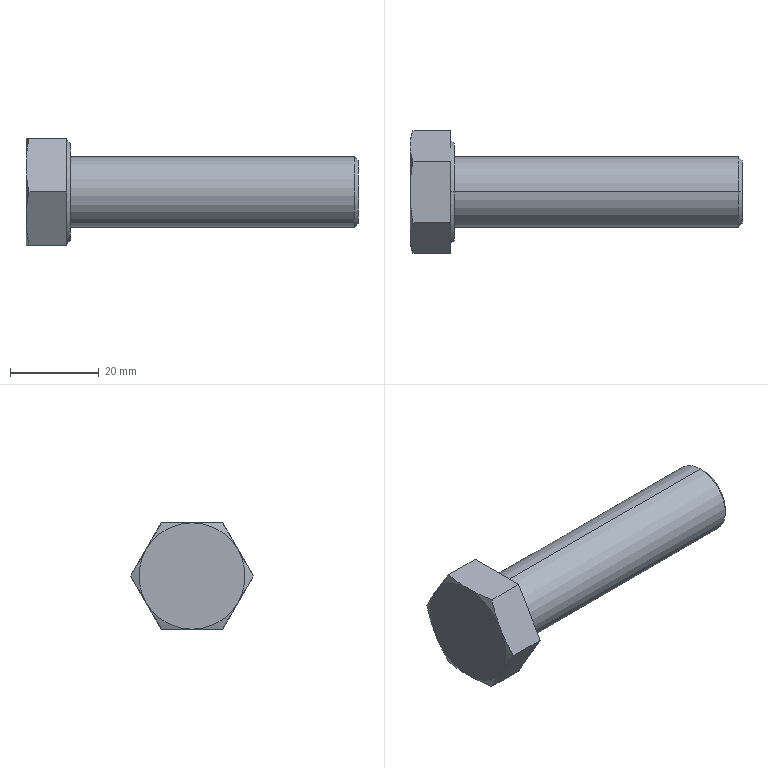Part | SolidWorks | features RevCut 3, Boss 1, Chamfer 1, Extrusion 1, Fillet 1, LPattern 1 | 1 solid | 22 faces | box 75 x 27.713 x 24 mm | volume 17960 mm3 | cone 10 | plane 10 | cylinder 2 | commonest cylinder face diameters 16 x2
STEP:
#1=CARTESIAN_POINT('',(75.,0.,-7.2));
#2=VERTEX_POINT('',#1);
#3=CARTESIAN_POINT('',(75.,0.,7.2));
#4=VERTEX_POINT('',#3);
#5=CARTESIAN_POINT('',(75.,0.,0.));
#6=DIRECTION('',(1.,0.,0.));
#7=DIRECTION('',(0.,0.,-1.));
#8=AXIS2_PLACEMENT_3D('',#5,#6,#7);
#9=CIRCLE('',#8,7.2);
#10=EDGE_CURVE('',#2,#4,#9,.T.);
#11=ORIENTED_EDGE('',*,*,#10,.F.);
#12=CARTESIAN_POINT('',(74.2,0.,-8.));
#13=VERTEX_POINT('',#12);
#14=CARTESIAN_POINT('',(75.,0.,-7.2));
#15=DIRECTION('',(-0.7071,0.,-0.7071));
#16=VECTOR('',#15,1000.);
#17=LINE('',#14,#16);
#18=EDGE_CURVE('',#2,#13,#17,.T.);
#19=ORIENTED_EDGE('',*,*,#18,.T.);
#20=CARTESIAN_POINT('',(74.2,0.,8.));
#21=VERTEX_POINT('',#20);
#22=CARTESIAN_POINT('',(74.2,0.,0.));
#23=DIRECTION('',(-1.,0.,0.));
#24=DIRECTION('',(0.,0.,-1.));
#25=AXIS2_PLACEMENT_3D('',#22,#23,#24);
#26=CIRCLE('',#25,8.);
#27=EDGE_CURVE('',#21,#13,#26,.T.);
#28=ORIENTED_EDGE('',*,*,#27,.F.);
#29=CARTESIAN_POINT('',(75.,0.,7.2));
#30=DIRECTION('',(-0.7071,0.,0.7071));
#31=VECTOR('',#30,1000.);
#32=LINE('',#29,#31);
#33=EDGE_CURVE('',#4,#21,#32,.T.);
#34=ORIENTED_EDGE('',*,*,#33,.F.);
#35=EDGE_LOOP('',(#11,#19,#28,#34));
#36=FACE_OUTER_BOUND('',#35,.T.);
#37=CARTESIAN_POINT('',(75.,0.,0.));
#38=DIRECTION('',(-1.,0.,0.));
#39=DIRECTION('',(0.,0.,1.));
#40=AXIS2_PLACEMENT_3D('',#37,#38,#39);
#41=CONICAL_SURFACE('',#40,7.2,0.7854);
#42=ADVANCED_FACE('',(#36),#41,.T.);
#43=ORIENTED_EDGE('',*,*,#27,.T.);
#44=CARTESIAN_POINT('',(10.,0.,-8.));
#45=VERTEX_POINT('',#44);
#46=CARTESIAN_POINT('',(75.,0.,-8.));
#47=DIRECTION('',(-1.,0.,0.));
#48=VECTOR('',#47,1000.);
#49=LINE('',#46,#48);
#50=EDGE_CURVE('',#13,#45,#49,.T.);
#51=ORIENTED_EDGE('',*,*,#50,.T.);
#52=CARTESIAN_POINT('',(10.,0.,8.));
#53=VERTEX_POINT('',#52);
#54=CARTESIAN_POINT('',(10.,0.,0.));
#55=DIRECTION('',(1.,0.,0.));
#56=DIRECTION('',(0.,0.,-1.));
#57=AXIS2_PLACEMENT_3D('',#54,#55,#56);
#58=CIRCLE('',#57,8.);
#59=EDGE_CURVE('',#45,#53,#58,.T.);
#60=ORIENTED_EDGE('',*,*,#59,.T.);
#61=CARTESIAN_POINT('',(75.,0.,8.));
#62=DIRECTION('',(-1.,0.,0.));
#63=VECTOR('',#62,1000.);
#64=LINE('',#61,#63);
#65=EDGE_CURVE('',#21,#53,#64,.T.);
#66=ORIENTED_EDGE('',*,*,#65,.F.);
#67=EDGE_LOOP('',(#43,#51,#60,#66));
#68=FACE_OUTER_BOUND('',#67,.T.);
#69=CARTESIAN_POINT('',(75.,0.,0.));
#70=DIRECTION('',(-1.,0.,0.));
#71=DIRECTION('',(0.,0.,1.));
#72=AXIS2_PLACEMENT_3D('',#69,#70,#71);
#73=CYLINDRICAL_SURFACE('',#72,8.);
#74=ADVANCED_FACE('',(#68),#73,.T.);
#75=CARTESIAN_POINT('',(10.,0.,11.));
#76=VERTEX_POINT('',#75);
#77=CARTESIAN_POINT('',(10.,0.,-11.));
#78=VERTEX_POINT('',#77);
#79=CARTESIAN_POINT('',(10.,0.,0.));
#80=DIRECTION('',(-1.,0.,0.));
#81=DIRECTION('',(0.,0.,1.));
#82=AXIS2_PLACEMENT_3D('',#79,#80,#81);
#83=CIRCLE('',#82,11.);
#84=EDGE_CURVE('',#76,#78,#83,.T.);
#85=ORIENTED_EDGE('',*,*,#84,.T.);
#86=CARTESIAN_POINT('',(9.2,0.,-11.8));
#87=VERTEX_POINT('',#86);
#88=CARTESIAN_POINT('',(9.2,0.,-11.8));
#89=DIRECTION('',(-0.7071,0.,-0.7071));
#90=VECTOR('',#89,1000.);
#91=LINE('',#88,#90);
#92=EDGE_CURVE('',#78,#87,#91,.T.);
#93=ORIENTED_EDGE('',*,*,#92,.T.);
#94=CARTESIAN_POINT('',(9.2,0.,11.8));
#95=VERTEX_POINT('',#94);
#96=CARTESIAN_POINT('',(9.2,0.,0.));
#97=DIRECTION('',(-1.,0.,0.));
#98=DIRECTION('',(0.,0.,1.));
#99=AXIS2_PLACEMENT_3D('',#96,#97,#98);
#100=CIRCLE('',#99,11.8);
#101=EDGE_CURVE('',#95,#87,#100,.T.);
#102=ORIENTED_EDGE('',*,*,#101,.F.);
#103=CARTESIAN_POINT('',(9.2,0.,11.8));
#104=DIRECTION('',(-0.7071,0.,0.7071));
#105=VECTOR('',#104,1000.);
#106=LINE('',#103,#105);
#107=EDGE_CURVE('',#76,#95,#106,.T.);
#108=ORIENTED_EDGE('',*,*,#107,.F.);
#109=EDGE_LOOP('',(#85,#93,#102,#108));
#110=FACE_OUTER_BOUND('',#109,.T.);
#111=CARTESIAN_POINT('',(9.2,0.,0.));
#112=DIRECTION('',(-1.,0.,0.));
#113=DIRECTION('',(0.,0.,1.));
#114=AXIS2_PLACEMENT_3D('',#111,#112,#113);
#115=CONICAL_SURFACE('',#114,11.8,0.7854);
#116=ADVANCED_FACE('',(#110),#115,.T.);
#117=ORIENTED_EDGE('',*,*,#84,.F.);
#118=CARTESIAN_POINT('',(10.,0.,0.));
#119=DIRECTION('',(-1.,0.,0.));
#120=DIRECTION('',(0.,0.,1.));
#121=AXIS2_PLACEMENT_3D('',#118,#119,#120);
#122=CIRCLE('',#121,11.);
#123=EDGE_CURVE('',#78,#76,#122,.T.);
#124=ORIENTED_EDGE('',*,*,#123,.F.);
#125=EDGE_LOOP('',(#117,#124));
#126=FACE_OUTER_BOUND('',#125,.T.);
#127=CARTESIAN_POINT('',(10.,0.,0.));
#128=DIRECTION('',(1.,0.,0.));
#129=DIRECTION('',(0.,0.,-1.));
#130=AXIS2_PLACEMENT_3D('',#127,#128,#129);
#131=CIRCLE('',#130,8.);
#132=EDGE_CURVE('',#53,#45,#131,.T.);
#133=ORIENTED_EDGE('',*,*,#132,.F.);
#134=ORIENTED_EDGE('',*,*,#59,.F.);
#135=EDGE_LOOP('',(#133,#134));
#136=FACE_BOUND('',#135,.T.);
#137=CARTESIAN_POINT('',(10.,-20.785,-12.));
#138=DIRECTION('',(1.,0.,0.));
#139=DIRECTION('',(0.,0.,-1.));
#140=AXIS2_PLACEMENT_3D('',#137,#138,#139);
#141=PLANE('',#140);
#142=ADVANCED_FACE('',(#126,#136),#141,.T.);
#143=CARTESIAN_POINT('',(0.6757,-13.856,0.));
#144=VERTEX_POINT('',#143);
#145=CARTESIAN_POINT('',(0.,-10.392,6.));
#146=VERTEX_POINT('',#145);
#147=CARTESIAN_POINT('',(0.6757,-13.856,0.));
#148=CARTESIAN_POINT('',(0.4655,-13.279,1.));
#149=CARTESIAN_POINT('',(0.2949,-12.702,2.));
#150=CARTESIAN_POINT('',(0.06178,-11.547,4.));
#151=CARTESIAN_POINT('',(0.,-10.97,5.));
#152=CARTESIAN_POINT('',(0.,-10.392,6.));
#153=B_SPLINE_CURVE_WITH_KNOTS('',3,(#147,#148,#149,#150,#151,#152),.UNSPECIFIED.,.F.,.F.,(4,2,4),(0.000000231,0.003464,0.006928),.UNSPECIFIED.);
#154=EDGE_CURVE('',#144,#146,#153,.T.);
#155=ORIENTED_EDGE('',*,*,#154,.F.);
#156=CARTESIAN_POINT('',(9.2,-13.856,0.));
#157=VERTEX_POINT('',#156);
#158=CARTESIAN_POINT('',(10.,-13.856,0.));
#159=DIRECTION('',(-1.,0.,0.));
#160=VECTOR('',#159,1000.);
#161=LINE('',#158,#160);
#162=EDGE_CURVE('',#157,#144,#161,.T.);
#163=ORIENTED_EDGE('',*,*,#162,.F.);
#164=CARTESIAN_POINT('',(9.2,-6.928,12.));
#165=VERTEX_POINT('',#164);
#166=CARTESIAN_POINT('',(9.2,-6.928,12.));
#167=DIRECTION('',(0.,-0.5,-0.866));
#168=VECTOR('',#167,1000.);
#169=LINE('',#166,#168);
#170=EDGE_CURVE('',#165,#157,#169,.T.);
#171=ORIENTED_EDGE('',*,*,#170,.F.);
#172=CARTESIAN_POINT('',(0.6757,-6.928,12.));
#173=VERTEX_POINT('',#172);
#174=CARTESIAN_POINT('',(10.,-6.928,12.));
#175=DIRECTION('',(-1.,0.,0.));
#176=VECTOR('',#175,1000.);
#177=LINE('',#174,#176);
#178=EDGE_CURVE('',#165,#173,#177,.T.);
#179=ORIENTED_EDGE('',*,*,#178,.T.);
#180=CARTESIAN_POINT('',(0.,-10.392,6.));
#181=CARTESIAN_POINT('',(0.,-9.815,7.));
#182=CARTESIAN_POINT('',(0.06178,-9.238,8.));
#183=CARTESIAN_POINT('',(0.2949,-8.083,10.));
#184=CARTESIAN_POINT('',(0.4655,-7.506,11.));
#185=CARTESIAN_POINT('',(0.6757,-6.928,12.));
#186=B_SPLINE_CURVE_WITH_KNOTS('',3,(#180,#181,#182,#183,#184,#185),.UNSPECIFIED.,.F.,.F.,(4,2,4),(0.006928,0.01039,0.01386),.UNSPECIFIED.);
#187=EDGE_CURVE('',#146,#173,#186,.T.);
#188=ORIENTED_EDGE('',*,*,#187,.F.);
#189=EDGE_LOOP('',(#155,#163,#171,#179,#188));
#190=FACE_OUTER_BOUND('',#189,.T.);
#191=CARTESIAN_POINT('',(10.,-6.928,12.));
#192=DIRECTION('',(0.,0.866,-0.5));
#193=DIRECTION('',(0.,0.5,0.866));
#194=AXIS2_PLACEMENT_3D('',#191,#192,#193);
#195=PLANE('',#194);
#196=ADVANCED_FACE('',(#190),#195,.F.);
#197=CARTESIAN_POINT('',(0.6757,-6.928,-12.));
#198=VERTEX_POINT('',#197);
#199=CARTESIAN_POINT('',(0.,-10.392,-6.));
#200=VERTEX_POINT('',#199);
#201=CARTESIAN_POINT('',(0.6757,-6.928,-12.));
#202=CARTESIAN_POINT('',(0.4655,-7.506,-11.));
#203=CARTESIAN_POINT('',(0.2949,-8.083,-10.));
#204=CARTESIAN_POINT('',(0.06178,-9.238,-8.));
#205=CARTESIAN_POINT('',(0.,-9.815,-7.));
#206=CARTESIAN_POINT('',(0.,-10.392,-6.));
#207=B_SPLINE_CURVE_WITH_KNOTS('',3,(#201,#202,#203,#204,#205,#206),.UNSPECIFIED.,.F.,.F.,(4,2,4),(0.000000231,0.003464,0.006928),.UNSPECIFIED.);
#208=EDGE_CURVE('',#198,#200,#207,.T.);
#209=ORIENTED_EDGE('',*,*,#208,.F.);
#210=CARTESIAN_POINT('',(9.2,-6.928,-12.));
#211=VERTEX_POINT('',#210);
#212=CARTESIAN_POINT('',(10.,-6.928,-12.));
#213=DIRECTION('',(-1.,0.,0.));
#214=VECTOR('',#213,1000.);
#215=LINE('',#212,#214);
#216=EDGE_CURVE('',#211,#198,#215,.T.);
#217=ORIENTED_EDGE('',*,*,#216,.F.);
#218=CARTESIAN_POINT('',(9.2,-13.856,0.));
#219=DIRECTION('',(0.,0.5,-0.866));
#220=VECTOR('',#219,1000.);
#221=LINE('',#218,#220);
#222=EDGE_CURVE('',#157,#211,#221,.T.);
#223=ORIENTED_EDGE('',*,*,#222,.F.);
#224=ORIENTED_EDGE('',*,*,#162,.T.);
#225=CARTESIAN_POINT('',(0.,-10.392,-6.));
#226=CARTESIAN_POINT('',(0.,-10.97,-5.));
#227=CARTESIAN_POINT('',(0.06178,-11.547,-4.));
#228=CARTESIAN_POINT('',(0.2949,-12.702,-2.));
#229=CARTESIAN_POINT('',(0.4655,-13.279,-1.));
#230=CARTESIAN_POINT('',(0.6757,-13.856,0.));
#231=B_SPLINE_CURVE_WITH_KNOTS('',3,(#225,#226,#227,#228,#229,#230),.UNSPECIFIED.,.F.,.F.,(4,2,4),(0.006928,0.01039,0.01386),.UNSPECIFIED.);
#232=EDGE_CURVE('',#200,#144,#231,.T.);
#233=ORIENTED_EDGE('',*,*,#232,.F.);
#234=EDGE_LOOP('',(#209,#217,#223,#224,#233));
#235=FACE_OUTER_BOUND('',#234,.T.);
#236=CARTESIAN_POINT('',(10.,-13.856,0.));
#237=DIRECTION('',(0.,0.866,0.5));
#238=DIRECTION('',(0.,-0.5,0.866));
#239=AXIS2_PLACEMENT_3D('',#236,#237,#238);
#240=PLANE('',#239);
#241=ADVANCED_FACE('',(#235),#240,.F.);
#242=CARTESIAN_POINT('',(0.6757,6.928,-12.));
#243=VERTEX_POINT('',#242);
#244=CARTESIAN_POINT('',(0.,0.,-12.));
#245=VERTEX_POINT('',#244);
#246=CARTESIAN_POINT('',(0.6757,6.928,-12.));
#247=CARTESIAN_POINT('',(0.4661,5.777,-12.));
#248=CARTESIAN_POINT('',(0.2953,4.622,-12.));
#249=CARTESIAN_POINT('',(0.06203,2.313,-12.));
#250=CARTESIAN_POINT('',(0.,1.157,-12.));
#251=CARTESIAN_POINT('',(0.,0.,-12.));
#252=B_SPLINE_CURVE_WITH_KNOTS('',3,(#246,#247,#248,#249,#250,#251),.UNSPECIFIED.,.F.,.F.,(4,2,4),(0.02498,0.02848,0.03197),.UNSPECIFIED.);
#253=EDGE_CURVE('',#243,#245,#252,.T.);
#254=ORIENTED_EDGE('',*,*,#253,.F.);
#255=CARTESIAN_POINT('',(9.2,6.928,-12.));
#256=VERTEX_POINT('',#255);
#257=CARTESIAN_POINT('',(10.,6.928,-12.));
#258=DIRECTION('',(-1.,0.,0.));
#259=VECTOR('',#258,1000.);
#260=LINE('',#257,#259);
#261=EDGE_CURVE('',#256,#243,#260,.T.);
#262=ORIENTED_EDGE('',*,*,#261,.F.);
#263=CARTESIAN_POINT('',(9.2,-6.928,-12.));
#264=DIRECTION('',(0.,1.,0.));
#265=VECTOR('',#264,1000.);
#266=LINE('',#263,#265);
#267=EDGE_CURVE('',#211,#256,#266,.T.);
#268=ORIENTED_EDGE('',*,*,#267,.F.);
#269=ORIENTED_EDGE('',*,*,#216,.T.);
#270=CARTESIAN_POINT('',(0.,0.,-12.));
#271=CARTESIAN_POINT('',(0.,-1.154,-12.));
#272=CARTESIAN_POINT('',(0.06169,-2.309,-12.));
#273=CARTESIAN_POINT('',(0.2952,-4.621,-12.));
#274=CARTESIAN_POINT('',(0.4669,-5.781,-12.));
#275=CARTESIAN_POINT('',(0.6757,-6.928,-12.));
#276=B_SPLINE_CURVE_WITH_KNOTS('',3,(#270,#271,#272,#273,#274,#275),.UNSPECIFIED.,.F.,.F.,(4,2,4),(0.03197,0.03545,0.03893),.UNSPECIFIED.);
#277=EDGE_CURVE('',#245,#198,#276,.T.);
#278=ORIENTED_EDGE('',*,*,#277,.F.);
#279=EDGE_LOOP('',(#254,#262,#268,#269,#278));
#280=FACE_OUTER_BOUND('',#279,.T.);
#281=CARTESIAN_POINT('',(10.,-6.928,-12.));
#282=DIRECTION('',(0.,0.,1.));
#283=DIRECTION('',(0.,-1.,0.));
#284=AXIS2_PLACEMENT_3D('',#281,#282,#283);
#285=PLANE('',#284);
#286=ADVANCED_FACE('',(#280),#285,.F.);
#287=CARTESIAN_POINT('',(0.6757,13.856,0.));
#288=VERTEX_POINT('',#287);
#289=CARTESIAN_POINT('',(0.,10.392,-6.));
#290=VERTEX_POINT('',#289);
#291=CARTESIAN_POINT('',(0.6757,13.856,0.));
#292=CARTESIAN_POINT('',(0.4655,13.279,-1.));
#293=CARTESIAN_POINT('',(0.2949,12.702,-2.));
#294=CARTESIAN_POINT('',(0.06178,11.547,-4.));
#295=CARTESIAN_POINT('',(0.,10.97,-5.));
#296=CARTESIAN_POINT('',(0.,10.392,-6.));
#297=B_SPLINE_CURVE_WITH_KNOTS('',3,(#291,#292,#293,#294,#295,#296),.UNSPECIFIED.,.F.,.F.,(4,2,4),(0.000000231,0.003464,0.006928),.UNSPECIFIED.);
#298=EDGE_CURVE('',#288,#290,#297,.T.);
#299=ORIENTED_EDGE('',*,*,#298,.F.);
#300=CARTESIAN_POINT('',(9.2,13.856,0.));
#301=VERTEX_POINT('',#300);
#302=CARTESIAN_POINT('',(10.,13.856,0.));
#303=DIRECTION('',(-1.,0.,0.));
#304=VECTOR('',#303,1000.);
#305=LINE('',#302,#304);
#306=EDGE_CURVE('',#301,#288,#305,.T.);
#307=ORIENTED_EDGE('',*,*,#306,.F.);
#308=CARTESIAN_POINT('',(9.2,6.928,-12.));
#309=DIRECTION('',(0.,0.5,0.866));
#310=VECTOR('',#309,1000.);
#311=LINE('',#308,#310);
#312=EDGE_CURVE('',#256,#301,#311,.T.);
#313=ORIENTED_EDGE('',*,*,#312,.F.);
#314=ORIENTED_EDGE('',*,*,#261,.T.);
#315=CARTESIAN_POINT('',(0.,10.392,-6.));
#316=CARTESIAN_POINT('',(0.,9.815,-7.));
#317=CARTESIAN_POINT('',(0.06178,9.238,-8.));
#318=CARTESIAN_POINT('',(0.2949,8.083,-10.));
#319=CARTESIAN_POINT('',(0.4655,7.506,-11.));
#320=CARTESIAN_POINT('',(0.6757,6.928,-12.));
#321=B_SPLINE_CURVE_WITH_KNOTS('',3,(#315,#316,#317,#318,#319,#320),.UNSPECIFIED.,.F.,.F.,(4,2,4),(0.006928,0.01039,0.01386),.UNSPECIFIED.);
#322=EDGE_CURVE('',#290,#243,#321,.T.);
#323=ORIENTED_EDGE('',*,*,#322,.F.);
#324=EDGE_LOOP('',(#299,#307,#313,#314,#323));
#325=FACE_OUTER_BOUND('',#324,.T.);
#326=CARTESIAN_POINT('',(10.,6.928,-12.));
#327=DIRECTION('',(0.,-0.866,0.5));
#328=DIRECTION('',(0.,-0.5,-0.866));
#329=AXIS2_PLACEMENT_3D('',#326,#327,#328);
#330=PLANE('',#329);
#331=ADVANCED_FACE('',(#325),#330,.F.);
#332=CARTESIAN_POINT('',(0.6757,6.928,12.));
#333=VERTEX_POINT('',#332);
#334=CARTESIAN_POINT('',(0.,10.392,6.));
#335=VERTEX_POINT('',#334);
#336=CARTESIAN_POINT('',(0.6757,6.928,12.));
#337=CARTESIAN_POINT('',(0.4655,7.506,11.));
#338=CARTESIAN_POINT('',(0.2949,8.083,10.));
#339=CARTESIAN_POINT('',(0.06178,9.238,8.));
#340=CARTESIAN_POINT('',(0.,9.815,7.));
#341=CARTESIAN_POINT('',(0.,10.392,6.));
#342=B_SPLINE_CURVE_WITH_KNOTS('',3,(#336,#337,#338,#339,#340,#341),.UNSPECIFIED.,.F.,.F.,(4,2,4),(0.000000231,0.003464,0.006928),.UNSPECIFIED.);
#343=EDGE_CURVE('',#333,#335,#342,.T.);
#344=ORIENTED_EDGE('',*,*,#343,.F.);
#345=CARTESIAN_POINT('',(9.2,6.928,12.));
#346=VERTEX_POINT('',#345);
#347=CARTESIAN_POINT('',(10.,6.928,12.));
#348=DIRECTION('',(-1.,0.,0.));
#349=VECTOR('',#348,1000.);
#350=LINE('',#347,#349);
#351=EDGE_CURVE('',#346,#333,#350,.T.);
#352=ORIENTED_EDGE('',*,*,#351,.F.);
#353=CARTESIAN_POINT('',(9.2,13.856,0.));
#354=DIRECTION('',(0.,-0.5,0.866));
#355=VECTOR('',#354,1000.);
#356=LINE('',#353,#355);
#357=EDGE_CURVE('',#301,#346,#356,.T.);
#358=ORIENTED_EDGE('',*,*,#357,.F.);
#359=ORIENTED_EDGE('',*,*,#306,.T.);
#360=CARTESIAN_POINT('',(0.,10.392,6.));
#361=CARTESIAN_POINT('',(0.,10.97,5.));
#362=CARTESIAN_POINT('',(0.06178,11.547,4.));
#363=CARTESIAN_POINT('',(0.2949,12.702,2.));
#364=CARTESIAN_POINT('',(0.4655,13.279,1.));
#365=CARTESIAN_POINT('',(0.6757,13.856,0.));
#366=B_SPLINE_CURVE_WITH_KNOTS('',3,(#360,#361,#362,#363,#364,#365),.UNSPECIFIED.,.F.,.F.,(4,2,4),(0.006928,0.01039,0.01386),.UNSPECIFIED.);
#367=EDGE_CURVE('',#335,#288,#366,.T.);
#368=ORIENTED_EDGE('',*,*,#367,.F.);
#369=EDGE_LOOP('',(#344,#352,#358,#359,#368));
#370=FACE_OUTER_BOUND('',#369,.T.);
#371=CARTESIAN_POINT('',(10.,13.856,0.));
#372=DIRECTION('',(0.,-0.866,-0.5));
#373=DIRECTION('',(0.,0.5,-0.866));
#374=AXIS2_PLACEMENT_3D('',#371,#372,#373);
#375=PLANE('',#374);
#376=ADVANCED_FACE('',(#370),#375,.F.);
#377=CARTESIAN_POINT('',(0.,0.,12.));
#378=VERTEX_POINT('',#377);
#379=CARTESIAN_POINT('',(0.6757,-6.928,12.));
#380=CARTESIAN_POINT('',(0.4669,-5.781,12.));
#381=CARTESIAN_POINT('',(0.2952,-4.621,12.));
#382=CARTESIAN_POINT('',(0.06169,-2.309,12.));
#383=CARTESIAN_POINT('',(0.,-1.154,12.));
#384=CARTESIAN_POINT('',(0.,0.,12.));
#385=B_SPLINE_CURVE_WITH_KNOTS('',3,(#379,#380,#381,#382,#383,#384),.UNSPECIFIED.,.F.,.F.,(4,2,4),(0.01179,0.01528,0.01877),.UNSPECIFIED.);
#386=EDGE_CURVE('',#173,#378,#385,.T.);
#387=ORIENTED_EDGE('',*,*,#386,.F.);
#388=ORIENTED_EDGE('',*,*,#178,.F.);
#389=CARTESIAN_POINT('',(9.2,6.928,12.));
#390=DIRECTION('',(0.,-1.,0.));
#391=VECTOR('',#390,1000.);
#392=LINE('',#389,#391);
#393=EDGE_CURVE('',#346,#165,#392,.T.);
#394=ORIENTED_EDGE('',*,*,#393,.F.);
#395=ORIENTED_EDGE('',*,*,#351,.T.);
#396=CARTESIAN_POINT('',(0.,0.,12.));
#397=CARTESIAN_POINT('',(0.,1.157,12.));
#398=CARTESIAN_POINT('',(0.06203,2.313,12.));
#399=CARTESIAN_POINT('',(0.2953,4.622,12.));
#400=CARTESIAN_POINT('',(0.4661,5.777,12.));
#401=CARTESIAN_POINT('',(0.6757,6.928,12.));
#402=B_SPLINE_CURVE_WITH_KNOTS('',3,(#396,#397,#398,#399,#400,#401),.UNSPECIFIED.,.F.,.F.,(4,2,4),(0.01877,0.02227,0.02577),.UNSPECIFIED.);
#403=EDGE_CURVE('',#378,#333,#402,.T.);
#404=ORIENTED_EDGE('',*,*,#403,.F.);
#405=EDGE_LOOP('',(#387,#388,#394,#395,#404));
#406=FACE_OUTER_BOUND('',#405,.T.);
#407=CARTESIAN_POINT('',(10.,6.928,12.));
#408=DIRECTION('',(0.,0.,-1.));
#409=DIRECTION('',(-1.,0.,0.));
#410=AXIS2_PLACEMENT_3D('',#407,#408,#409);
#411=PLANE('',#410);
#412=ADVANCED_FACE('',(#406),#411,.F.);
#413=ORIENTED_EDGE('',*,*,#101,.T.);
#414=CARTESIAN_POINT('',(9.2,0.,0.));
#415=DIRECTION('',(-1.,0.,0.));
#416=DIRECTION('',(0.,0.,1.));
#417=AXIS2_PLACEMENT_3D('',#414,#415,#416);
#418=CIRCLE('',#417,11.8);
#419=EDGE_CURVE('',#87,#95,#418,.T.);
#420=ORIENTED_EDGE('',*,*,#419,.T.);
#421=EDGE_LOOP('',(#413,#420));
#422=FACE_BOUND('',#421,.T.);
#423=ORIENTED_EDGE('',*,*,#170,.T.);
#424=ORIENTED_EDGE('',*,*,#222,.T.);
#425=ORIENTED_EDGE('',*,*,#267,.T.);
#426=ORIENTED_EDGE('',*,*,#312,.T.);
#427=ORIENTED_EDGE('',*,*,#357,.T.);
#428=ORIENTED_EDGE('',*,*,#393,.T.);
#429=EDGE_LOOP('',(#423,#424,#425,#426,#427,#428));
#430=FACE_OUTER_BOUND('',#429,.T.);
#431=CARTESIAN_POINT('',(9.2,11.8,0.));
#432=DIRECTION('',(1.,0.,0.));
#433=DIRECTION('',(0.,0.,-1.));
#434=AXIS2_PLACEMENT_3D('',#431,#432,#433);
#435=PLANE('',#434);
#436=ADVANCED_FACE('',(#422,#430),#435,.T.);
#437=ORIENTED_EDGE('',*,*,#92,.F.);
#438=ORIENTED_EDGE('',*,*,#123,.T.);
#439=ORIENTED_EDGE('',*,*,#107,.T.);
#440=ORIENTED_EDGE('',*,*,#419,.F.);
#441=EDGE_LOOP('',(#437,#438,#439,#440));
#442=FACE_OUTER_BOUND('',#441,.T.);
#443=CARTESIAN_POINT('',(9.2,0.,0.));
#444=DIRECTION('',(-1.,0.,0.));
#445=DIRECTION('',(0.,0.,1.));
#446=AXIS2_PLACEMENT_3D('',#443,#444,#445);
#447=CONICAL_SURFACE('',#446,11.8,0.7854);
#448=ADVANCED_FACE('',(#442),#447,.T.);
#449=ORIENTED_EDGE('',*,*,#277,.T.);
#450=ORIENTED_EDGE('',*,*,#208,.T.);
#451=CARTESIAN_POINT('',(0.,0.,0.));
#452=DIRECTION('',(1.,0.,0.));
#453=DIRECTION('',(0.,0.,-1.));
#454=AXIS2_PLACEMENT_3D('',#451,#452,#453);
#455=CIRCLE('',#454,12.);
#456=EDGE_CURVE('',#200,#245,#455,.T.);
#457=ORIENTED_EDGE('',*,*,#456,.T.);
#458=EDGE_LOOP('',(#449,#450,#457));
#459=FACE_OUTER_BOUND('',#458,.T.);
#460=CARTESIAN_POINT('',(0.,0.,0.));
#461=DIRECTION('',(1.,0.,0.));
#462=DIRECTION('',(0.,0.,-1.));
#463=AXIS2_PLACEMENT_3D('',#460,#461,#462);
#464=CONICAL_SURFACE('',#463,12.,1.222);
#465=ADVANCED_FACE('',(#459),#464,.T.);
#466=ORIENTED_EDGE('',*,*,#232,.T.);
#467=ORIENTED_EDGE('',*,*,#154,.T.);
#468=CARTESIAN_POINT('',(0.,0.,0.));
#469=DIRECTION('',(1.,0.,0.));
#470=DIRECTION('',(0.,0.,-1.));
#471=AXIS2_PLACEMENT_3D('',#468,#469,#470);
#472=CIRCLE('',#471,12.);
#473=EDGE_CURVE('',#146,#200,#472,.T.);
#474=ORIENTED_EDGE('',*,*,#473,.T.);
#475=EDGE_LOOP('',(#466,#467,#474));
#476=FACE_OUTER_BOUND('',#475,.T.);
#477=CARTESIAN_POINT('',(0.,0.,0.));
#478=DIRECTION('',(1.,0.,0.));
#479=DIRECTION('',(0.,0.,-1.));
#480=AXIS2_PLACEMENT_3D('',#477,#478,#479);
#481=CONICAL_SURFACE('',#480,12.,1.222);
#482=ADVANCED_FACE('',(#476),#481,.T.);
#483=ORIENTED_EDGE('',*,*,#187,.T.);
#484=ORIENTED_EDGE('',*,*,#386,.T.);
#485=CARTESIAN_POINT('',(0.,0.,0.));
#486=DIRECTION('',(1.,0.,0.));
#487=DIRECTION('',(0.,0.,-1.));
#488=AXIS2_PLACEMENT_3D('',#485,#486,#487);
#489=CIRCLE('',#488,12.);
#490=EDGE_CURVE('',#378,#146,#489,.T.);
#491=ORIENTED_EDGE('',*,*,#490,.T.);
#492=EDGE_LOOP('',(#483,#484,#491));
#493=FACE_OUTER_BOUND('',#492,.T.);
#494=CARTESIAN_POINT('',(0.,0.,0.));
#495=DIRECTION('',(1.,0.,0.));
#496=DIRECTION('',(0.,0.,-1.));
#497=AXIS2_PLACEMENT_3D('',#494,#495,#496);
#498=CONICAL_SURFACE('',#497,12.,1.222);
#499=ADVANCED_FACE('',(#493),#498,.T.);
#500=ORIENTED_EDGE('',*,*,#343,.T.);
#501=CARTESIAN_POINT('',(0.,0.,0.));
#502=DIRECTION('',(-1.,0.,0.));
#503=DIRECTION('',(0.,0.,1.));
#504=AXIS2_PLACEMENT_3D('',#501,#502,#503);
#505=CIRCLE('',#504,12.);
#506=EDGE_CURVE('',#378,#335,#505,.T.);
#507=ORIENTED_EDGE('',*,*,#506,.F.);
#508=ORIENTED_EDGE('',*,*,#403,.T.);
#509=EDGE_LOOP('',(#500,#507,#508));
#510=FACE_OUTER_BOUND('',#509,.T.);
#511=CARTESIAN_POINT('',(0.,0.,0.));
#512=DIRECTION('',(1.,0.,0.));
#513=DIRECTION('',(0.,0.,-1.));
#514=AXIS2_PLACEMENT_3D('',#511,#512,#513);
#515=CONICAL_SURFACE('',#514,12.,1.222);
#516=ADVANCED_FACE('',(#510),#515,.T.);
#517=ORIENTED_EDGE('',*,*,#298,.T.);
#518=CARTESIAN_POINT('',(0.,0.,0.));
#519=DIRECTION('',(1.,0.,0.));
#520=DIRECTION('',(0.,0.,-1.));
#521=AXIS2_PLACEMENT_3D('',#518,#519,#520);
#522=CIRCLE('',#521,12.);
#523=EDGE_CURVE('',#290,#335,#522,.T.);
#524=ORIENTED_EDGE('',*,*,#523,.T.);
#525=ORIENTED_EDGE('',*,*,#367,.T.);
#526=EDGE_LOOP('',(#517,#524,#525));
#527=FACE_OUTER_BOUND('',#526,.T.);
#528=CARTESIAN_POINT('',(0.,0.,0.));
#529=DIRECTION('',(1.,0.,0.));
#530=DIRECTION('',(0.,0.,-1.));
#531=AXIS2_PLACEMENT_3D('',#528,#529,#530);
#532=CONICAL_SURFACE('',#531,12.,1.222);
#533=ADVANCED_FACE('',(#527),#532,.T.);
#534=ORIENTED_EDGE('',*,*,#253,.T.);
#535=CARTESIAN_POINT('',(0.,0.,0.));
#536=DIRECTION('',(1.,0.,0.));
#537=DIRECTION('',(0.,0.,-1.));
#538=AXIS2_PLACEMENT_3D('',#535,#536,#537);
#539=CIRCLE('',#538,12.);
#540=EDGE_CURVE('',#245,#290,#539,.T.);
#541=ORIENTED_EDGE('',*,*,#540,.T.);
#542=ORIENTED_EDGE('',*,*,#322,.T.);
#543=EDGE_LOOP('',(#534,#541,#542));
#544=FACE_OUTER_BOUND('',#543,.T.);
#545=CARTESIAN_POINT('',(0.,0.,0.));
#546=DIRECTION('',(1.,0.,0.));
#547=DIRECTION('',(0.,0.,-1.));
#548=AXIS2_PLACEMENT_3D('',#545,#546,#547);
#549=CONICAL_SURFACE('',#548,12.,1.222);
#550=ADVANCED_FACE('',(#544),#549,.T.);
#551=ORIENTED_EDGE('',*,*,#540,.F.);
#552=ORIENTED_EDGE('',*,*,#456,.F.);
#553=ORIENTED_EDGE('',*,*,#473,.F.);
#554=ORIENTED_EDGE('',*,*,#490,.F.);
#555=ORIENTED_EDGE('',*,*,#506,.T.);
#556=ORIENTED_EDGE('',*,*,#523,.F.);
#557=EDGE_LOOP('',(#551,#552,#553,#554,#555,#556));
#558=FACE_OUTER_BOUND('',#557,.T.);
#559=CARTESIAN_POINT('',(0.,-20.785,-12.));
#560=DIRECTION('',(1.,0.,0.));
#561=DIRECTION('',(0.,0.,-1.));
#562=AXIS2_PLACEMENT_3D('',#559,#560,#561);
#563=PLANE('',#562);
#564=ADVANCED_FACE('',(#558),#563,.F.);
#565=ORIENTED_EDGE('',*,*,#50,.F.);
#566=CARTESIAN_POINT('',(74.2,0.,0.));
#567=DIRECTION('',(-1.,0.,0.));
#568=DIRECTION('',(0.,0.,-1.));
#569=AXIS2_PLACEMENT_3D('',#566,#567,#568);
#570=CIRCLE('',#569,8.);
#571=EDGE_CURVE('',#13,#21,#570,.T.);
#572=ORIENTED_EDGE('',*,*,#571,.T.);
#573=ORIENTED_EDGE('',*,*,#65,.T.);
#574=ORIENTED_EDGE('',*,*,#132,.T.);
#575=EDGE_LOOP('',(#565,#572,#573,#574));
#576=FACE_OUTER_BOUND('',#575,.T.);
#577=CARTESIAN_POINT('',(75.,0.,0.));
#578=DIRECTION('',(-1.,0.,0.));
#579=DIRECTION('',(0.,0.,1.));
#580=AXIS2_PLACEMENT_3D('',#577,#578,#579);
#581=CYLINDRICAL_SURFACE('',#580,8.);
#582=ADVANCED_FACE('',(#576),#581,.T.);
#583=CARTESIAN_POINT('',(75.,0.,0.));
#584=DIRECTION('',(1.,0.,0.));
#585=DIRECTION('',(0.,0.,-1.));
#586=AXIS2_PLACEMENT_3D('',#583,#584,#585);
#587=CIRCLE('',#586,7.2);
#588=EDGE_CURVE('',#4,#2,#587,.T.);
#589=ORIENTED_EDGE('',*,*,#588,.T.);
#590=ORIENTED_EDGE('',*,*,#10,.T.);
#591=EDGE_LOOP('',(#589,#590));
#592=FACE_OUTER_BOUND('',#591,.T.);
#593=CARTESIAN_POINT('',(75.,0.,0.));
#594=DIRECTION('',(1.,0.,0.));
#595=DIRECTION('',(0.,0.,-1.));
#596=AXIS2_PLACEMENT_3D('',#593,#594,#595);
#597=PLANE('',#596);
#598=ADVANCED_FACE('',(#592),#597,.T.);
#599=ORIENTED_EDGE('',*,*,#18,.F.);
#600=ORIENTED_EDGE('',*,*,#588,.F.);
#601=ORIENTED_EDGE('',*,*,#33,.T.);
#602=ORIENTED_EDGE('',*,*,#571,.F.);
#603=EDGE_LOOP('',(#599,#600,#601,#602));
#604=FACE_OUTER_BOUND('',#603,.T.);
#605=CARTESIAN_POINT('',(75.,0.,0.));
#606=DIRECTION('',(-1.,0.,0.));
#607=DIRECTION('',(0.,0.,1.));
#608=AXIS2_PLACEMENT_3D('',#605,#606,#607);
#609=CONICAL_SURFACE('',#608,7.2,0.7854);
#610=ADVANCED_FACE('',(#604),#609,.T.);
#611=CLOSED_SHELL('',(#42,#74,#116,#142,#196,#241,#286,#331,#376,#412,#436,#448,#465,#482,#499,#516,#533,#550,#564,#582,#598,#610));
#612=MANIFOLD_SOLID_BREP('',#611);
#613=CARTESIAN_POINT('',(0.,0.,0.));
#614=DIRECTION('',(0.,0.,1.));
#615=DIRECTION('',(1.,0.,0.));
#616=AXIS2_PLACEMENT_3D('',#613,#614,#615);
#617=(LENGTH_UNIT()NAMED_UNIT(*)SI_UNIT(.MILLI.,.METRE.));
#618=UNCERTAINTY_MEASURE_WITH_UNIT(LENGTH_MEASURE(0.00001),#617,'','');
#619=(NAMED_UNIT(*)PLANE_ANGLE_UNIT()SI_UNIT($,.RADIAN.));
#620=(NAMED_UNIT(*)SI_UNIT($,.STERADIAN.)SOLID_ANGLE_UNIT());
#621=(GEOMETRIC_REPRESENTATION_CONTEXT(3)GLOBAL_UNCERTAINTY_ASSIGNED_CONTEXT((#618))GLOBAL_UNIT_ASSIGNED_CONTEXT((#617,#619,#620))REPRESENTATION_CONTEXT('',''));
#622=ADVANCED_BREP_SHAPE_REPRESENTATION('',(#612,#616),#621);